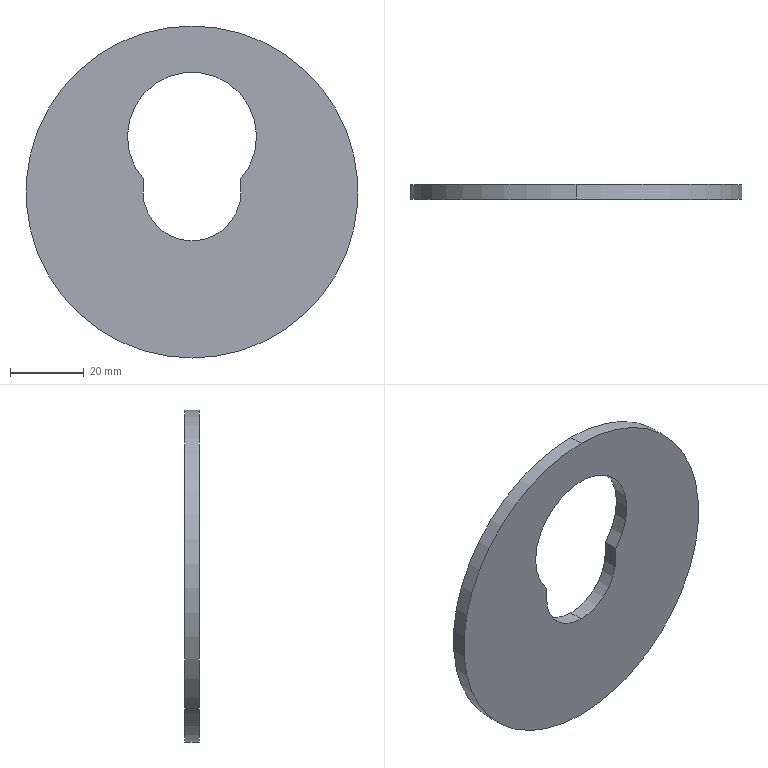Part | SolidWorks | features Extrusion 1, ICE 1 | 1 solid | 9 faces | box 90 x 4 x 90 mm | volume 20564 mm3 | cylinder 5 | plane 4 | commonest cylinder face diameters 26.5 x2 90 x2 35 x1
STEP:
#1=CARTESIAN_POINT('',(13.238,2.,0.5547));
#2=VERTEX_POINT('',#1);
#3=CARTESIAN_POINT('',(0.,2.,-13.25));
#4=VERTEX_POINT('',#3);
#5=CARTESIAN_POINT('',(0.,2.,0.));
#6=DIRECTION('',(0.,1.,0.));
#7=DIRECTION('',(0.,0.,1.));
#8=AXIS2_PLACEMENT_3D('',#5,#6,#7);
#9=CIRCLE('',#8,13.25);
#10=EDGE_CURVE('',#2,#4,#9,.T.);
#11=ORIENTED_EDGE('',*,*,#10,.T.);
#12=CARTESIAN_POINT('',(0.,-2.,-13.25));
#13=VERTEX_POINT('',#12);
#14=CARTESIAN_POINT('',(0.,2.,-13.25));
#15=DIRECTION('',(0.,-1.,0.));
#16=VECTOR('',#15,1000.);
#17=LINE('',#14,#16);
#18=EDGE_CURVE('',#4,#13,#17,.T.);
#19=ORIENTED_EDGE('',*,*,#18,.T.);
#20=CARTESIAN_POINT('',(13.238,-2.,0.5547));
#21=VERTEX_POINT('',#20);
#22=CARTESIAN_POINT('',(0.,-2.,0.));
#23=DIRECTION('',(0.,1.,0.));
#24=DIRECTION('',(0.,0.,1.));
#25=AXIS2_PLACEMENT_3D('',#22,#23,#24);
#26=CIRCLE('',#25,13.25);
#27=EDGE_CURVE('',#21,#13,#26,.T.);
#28=ORIENTED_EDGE('',*,*,#27,.F.);
#29=CARTESIAN_POINT('',(13.238,2.,0.5547));
#30=DIRECTION('',(0.,1.,0.));
#31=VECTOR('',#30,1000.);
#32=LINE('',#29,#31);
#33=EDGE_CURVE('',#21,#2,#32,.T.);
#34=ORIENTED_EDGE('',*,*,#33,.T.);
#35=EDGE_LOOP('',(#11,#19,#28,#34));
#36=FACE_OUTER_BOUND('',#35,.T.);
#37=CARTESIAN_POINT('',(0.,2.,0.));
#38=DIRECTION('',(0.,-1.,0.));
#39=DIRECTION('',(0.,0.,-1.));
#40=AXIS2_PLACEMENT_3D('',#37,#38,#39);
#41=CYLINDRICAL_SURFACE('',#40,13.25);
#42=ADVANCED_FACE('',(#36),#41,.F.);
#43=CARTESIAN_POINT('',(0.,2.,45.));
#44=VERTEX_POINT('',#43);
#45=CARTESIAN_POINT('',(0.,2.,-45.));
#46=VERTEX_POINT('',#45);
#47=CARTESIAN_POINT('',(0.,2.,0.));
#48=DIRECTION('',(0.,1.,0.));
#49=DIRECTION('',(0.,0.,1.));
#50=AXIS2_PLACEMENT_3D('',#47,#48,#49);
#51=CIRCLE('',#50,45.);
#52=EDGE_CURVE('',#44,#46,#51,.T.);
#53=ORIENTED_EDGE('',*,*,#52,.F.);
#54=CARTESIAN_POINT('',(0.,-2.,45.));
#55=VERTEX_POINT('',#54);
#56=CARTESIAN_POINT('',(0.,2.,45.));
#57=DIRECTION('',(0.,-1.,0.));
#58=VECTOR('',#57,1000.);
#59=LINE('',#56,#58);
#60=EDGE_CURVE('',#44,#55,#59,.T.);
#61=ORIENTED_EDGE('',*,*,#60,.T.);
#62=CARTESIAN_POINT('',(0.,-2.,-45.));
#63=VERTEX_POINT('',#62);
#64=CARTESIAN_POINT('',(0.,-2.,0.));
#65=DIRECTION('',(0.,1.,0.));
#66=DIRECTION('',(0.,0.,1.));
#67=AXIS2_PLACEMENT_3D('',#64,#65,#66);
#68=CIRCLE('',#67,45.);
#69=EDGE_CURVE('',#55,#63,#68,.T.);
#70=ORIENTED_EDGE('',*,*,#69,.T.);
#71=CARTESIAN_POINT('',(0.,2.,-45.));
#72=DIRECTION('',(0.,-1.,0.));
#73=VECTOR('',#72,1000.);
#74=LINE('',#71,#73);
#75=EDGE_CURVE('',#46,#63,#74,.T.);
#76=ORIENTED_EDGE('',*,*,#75,.F.);
#77=EDGE_LOOP('',(#53,#61,#70,#76));
#78=FACE_OUTER_BOUND('',#77,.T.);
#79=CARTESIAN_POINT('',(0.,2.,0.));
#80=DIRECTION('',(0.,-1.,0.));
#81=DIRECTION('',(0.,0.,-1.));
#82=AXIS2_PLACEMENT_3D('',#79,#80,#81);
#83=CYLINDRICAL_SURFACE('',#82,45.);
#84=ADVANCED_FACE('',(#78),#83,.T.);
#85=CARTESIAN_POINT('',(13.238,2.,3.555));
#86=VERTEX_POINT('',#85);
#87=CARTESIAN_POINT('',(13.238,2.,0.5547));
#88=DIRECTION('',(0.,0.,1.));
#89=VECTOR('',#88,1000.);
#90=LINE('',#87,#89);
#91=EDGE_CURVE('',#2,#86,#90,.T.);
#92=ORIENTED_EDGE('',*,*,#91,.T.);
#93=CARTESIAN_POINT('',(-13.238,2.,3.555));
#94=VERTEX_POINT('',#93);
#95=CARTESIAN_POINT('',(0.,2.,15.));
#96=DIRECTION('',(0.,-1.,0.));
#97=DIRECTION('',(0.,0.,1.));
#98=AXIS2_PLACEMENT_3D('',#95,#96,#97);
#99=CIRCLE('',#98,17.5);
#100=EDGE_CURVE('',#86,#94,#99,.T.);
#101=ORIENTED_EDGE('',*,*,#100,.T.);
#102=CARTESIAN_POINT('',(-13.238,2.,0.5547));
#103=VERTEX_POINT('',#102);
#104=CARTESIAN_POINT('',(-13.238,2.,0.5547));
#105=DIRECTION('',(0.,0.,-1.));
#106=VECTOR('',#105,1000.);
#107=LINE('',#104,#106);
#108=EDGE_CURVE('',#94,#103,#107,.T.);
#109=ORIENTED_EDGE('',*,*,#108,.T.);
#110=CARTESIAN_POINT('',(0.,2.,0.));
#111=DIRECTION('',(0.,1.,0.));
#112=DIRECTION('',(0.,0.,1.));
#113=AXIS2_PLACEMENT_3D('',#110,#111,#112);
#114=CIRCLE('',#113,13.25);
#115=EDGE_CURVE('',#4,#103,#114,.T.);
#116=ORIENTED_EDGE('',*,*,#115,.F.);
#117=ORIENTED_EDGE('',*,*,#10,.F.);
#118=EDGE_LOOP('',(#92,#101,#109,#116,#117));
#119=FACE_BOUND('',#118,.T.);
#120=CARTESIAN_POINT('',(0.,2.,0.));
#121=DIRECTION('',(0.,1.,0.));
#122=DIRECTION('',(0.,0.,1.));
#123=AXIS2_PLACEMENT_3D('',#120,#121,#122);
#124=CIRCLE('',#123,45.);
#125=EDGE_CURVE('',#46,#44,#124,.T.);
#126=ORIENTED_EDGE('',*,*,#125,.T.);
#127=ORIENTED_EDGE('',*,*,#52,.T.);
#128=EDGE_LOOP('',(#126,#127));
#129=FACE_OUTER_BOUND('',#128,.T.);
#130=CARTESIAN_POINT('',(0.,2.,0.));
#131=DIRECTION('',(0.,1.,0.));
#132=DIRECTION('',(0.,0.,1.));
#133=AXIS2_PLACEMENT_3D('',#130,#131,#132);
#134=PLANE('',#133);
#135=ADVANCED_FACE('',(#119,#129),#134,.T.);
#136=CARTESIAN_POINT('',(0.,-2.,0.));
#137=DIRECTION('',(0.,1.,0.));
#138=DIRECTION('',(0.,0.,1.));
#139=AXIS2_PLACEMENT_3D('',#136,#137,#138);
#140=CIRCLE('',#139,45.);
#141=EDGE_CURVE('',#63,#55,#140,.T.);
#142=ORIENTED_EDGE('',*,*,#141,.F.);
#143=ORIENTED_EDGE('',*,*,#69,.F.);
#144=EDGE_LOOP('',(#142,#143));
#145=FACE_OUTER_BOUND('',#144,.T.);
#146=CARTESIAN_POINT('',(13.238,-2.,3.555));
#147=VERTEX_POINT('',#146);
#148=CARTESIAN_POINT('',(-13.238,-2.,3.555));
#149=VERTEX_POINT('',#148);
#150=CARTESIAN_POINT('',(0.,-2.,15.));
#151=DIRECTION('',(0.,-1.,0.));
#152=DIRECTION('',(0.,0.,-1.));
#153=AXIS2_PLACEMENT_3D('',#150,#151,#152);
#154=CIRCLE('',#153,17.5);
#155=EDGE_CURVE('',#147,#149,#154,.T.);
#156=ORIENTED_EDGE('',*,*,#155,.F.);
#157=CARTESIAN_POINT('',(13.238,-2.,0.5547));
#158=DIRECTION('',(0.,0.,1.));
#159=VECTOR('',#158,1000.);
#160=LINE('',#157,#159);
#161=EDGE_CURVE('',#21,#147,#160,.T.);
#162=ORIENTED_EDGE('',*,*,#161,.F.);
#163=ORIENTED_EDGE('',*,*,#27,.T.);
#164=CARTESIAN_POINT('',(-13.238,-2.,0.5547));
#165=VERTEX_POINT('',#164);
#166=CARTESIAN_POINT('',(0.,-2.,0.));
#167=DIRECTION('',(0.,1.,0.));
#168=DIRECTION('',(0.,0.,1.));
#169=AXIS2_PLACEMENT_3D('',#166,#167,#168);
#170=CIRCLE('',#169,13.25);
#171=EDGE_CURVE('',#13,#165,#170,.T.);
#172=ORIENTED_EDGE('',*,*,#171,.T.);
#173=CARTESIAN_POINT('',(-13.238,-2.,0.5547));
#174=DIRECTION('',(0.,0.,-1.));
#175=VECTOR('',#174,1000.);
#176=LINE('',#173,#175);
#177=EDGE_CURVE('',#149,#165,#176,.T.);
#178=ORIENTED_EDGE('',*,*,#177,.F.);
#179=EDGE_LOOP('',(#156,#162,#163,#172,#178));
#180=FACE_BOUND('',#179,.T.);
#181=CARTESIAN_POINT('',(0.,-2.,0.));
#182=DIRECTION('',(0.,1.,0.));
#183=DIRECTION('',(0.,0.,1.));
#184=AXIS2_PLACEMENT_3D('',#181,#182,#183);
#185=PLANE('',#184);
#186=ADVANCED_FACE('',(#145,#180),#185,.F.);
#187=ORIENTED_EDGE('',*,*,#60,.F.);
#188=ORIENTED_EDGE('',*,*,#125,.F.);
#189=ORIENTED_EDGE('',*,*,#75,.T.);
#190=ORIENTED_EDGE('',*,*,#141,.T.);
#191=EDGE_LOOP('',(#187,#188,#189,#190));
#192=FACE_OUTER_BOUND('',#191,.T.);
#193=CARTESIAN_POINT('',(0.,2.,0.));
#194=DIRECTION('',(0.,-1.,0.));
#195=DIRECTION('',(0.,0.,-1.));
#196=AXIS2_PLACEMENT_3D('',#193,#194,#195);
#197=CYLINDRICAL_SURFACE('',#196,45.);
#198=ADVANCED_FACE('',(#192),#197,.T.);
#199=ORIENTED_EDGE('',*,*,#18,.F.);
#200=ORIENTED_EDGE('',*,*,#115,.T.);
#201=CARTESIAN_POINT('',(-13.238,2.,0.5547));
#202=DIRECTION('',(0.,-1.,0.));
#203=VECTOR('',#202,1000.);
#204=LINE('',#201,#203);
#205=EDGE_CURVE('',#103,#165,#204,.T.);
#206=ORIENTED_EDGE('',*,*,#205,.T.);
#207=ORIENTED_EDGE('',*,*,#171,.F.);
#208=EDGE_LOOP('',(#199,#200,#206,#207));
#209=FACE_OUTER_BOUND('',#208,.T.);
#210=CARTESIAN_POINT('',(0.,2.,0.));
#211=DIRECTION('',(0.,-1.,0.));
#212=DIRECTION('',(0.,0.,-1.));
#213=AXIS2_PLACEMENT_3D('',#210,#211,#212);
#214=CYLINDRICAL_SURFACE('',#213,13.25);
#215=ADVANCED_FACE('',(#209),#214,.F.);
#216=CARTESIAN_POINT('',(13.238,2.001,3.555));
#217=DIRECTION('',(0.,-1.,0.));
#218=VECTOR('',#217,1000.);
#219=LINE('',#216,#218);
#220=EDGE_CURVE('',#86,#147,#219,.T.);
#221=ORIENTED_EDGE('',*,*,#220,.T.);
#222=ORIENTED_EDGE('',*,*,#155,.T.);
#223=CARTESIAN_POINT('',(-13.238,2.001,3.555));
#224=DIRECTION('',(0.,-1.,0.));
#225=VECTOR('',#224,1000.);
#226=LINE('',#223,#225);
#227=EDGE_CURVE('',#94,#149,#226,.T.);
#228=ORIENTED_EDGE('',*,*,#227,.F.);
#229=ORIENTED_EDGE('',*,*,#100,.F.);
#230=EDGE_LOOP('',(#221,#222,#228,#229));
#231=FACE_OUTER_BOUND('',#230,.T.);
#232=CARTESIAN_POINT('',(0.,2.001,15.));
#233=DIRECTION('',(0.,-1.,0.));
#234=DIRECTION('',(0.,0.,-1.));
#235=AXIS2_PLACEMENT_3D('',#232,#233,#234);
#236=CYLINDRICAL_SURFACE('',#235,17.5);
#237=ADVANCED_FACE('',(#231),#236,.F.);
#238=ORIENTED_EDGE('',*,*,#33,.F.);
#239=ORIENTED_EDGE('',*,*,#161,.T.);
#240=ORIENTED_EDGE('',*,*,#220,.F.);
#241=ORIENTED_EDGE('',*,*,#91,.F.);
#242=EDGE_LOOP('',(#238,#239,#240,#241));
#243=FACE_OUTER_BOUND('',#242,.T.);
#244=CARTESIAN_POINT('',(13.238,2.001,0.5547));
#245=DIRECTION('',(1.,0.,0.));
#246=DIRECTION('',(0.,0.,-1.));
#247=AXIS2_PLACEMENT_3D('',#244,#245,#246);
#248=PLANE('',#247);
#249=ADVANCED_FACE('',(#243),#248,.F.);
#250=ORIENTED_EDGE('',*,*,#227,.T.);
#251=ORIENTED_EDGE('',*,*,#177,.T.);
#252=ORIENTED_EDGE('',*,*,#205,.F.);
#253=ORIENTED_EDGE('',*,*,#108,.F.);
#254=EDGE_LOOP('',(#250,#251,#252,#253));
#255=FACE_OUTER_BOUND('',#254,.T.);
#256=CARTESIAN_POINT('',(-13.238,2.001,0.5547));
#257=DIRECTION('',(-1.,0.,0.));
#258=DIRECTION('',(0.,0.,1.));
#259=AXIS2_PLACEMENT_3D('',#256,#257,#258);
#260=PLANE('',#259);
#261=ADVANCED_FACE('',(#255),#260,.F.);
#262=CLOSED_SHELL('',(#42,#84,#135,#186,#198,#215,#237,#249,#261));
#263=MANIFOLD_SOLID_BREP('',#262);
#264=CARTESIAN_POINT('',(0.,0.,0.));
#265=DIRECTION('',(0.,0.,1.));
#266=DIRECTION('',(1.,0.,0.));
#267=AXIS2_PLACEMENT_3D('',#264,#265,#266);
#268=(LENGTH_UNIT()NAMED_UNIT(*)SI_UNIT(.MILLI.,.METRE.));
#269=UNCERTAINTY_MEASURE_WITH_UNIT(LENGTH_MEASURE(0.00001),#268,'','');
#270=(NAMED_UNIT(*)PLANE_ANGLE_UNIT()SI_UNIT($,.RADIAN.));
#271=(NAMED_UNIT(*)SI_UNIT($,.STERADIAN.)SOLID_ANGLE_UNIT());
#272=(GEOMETRIC_REPRESENTATION_CONTEXT(3)GLOBAL_UNCERTAINTY_ASSIGNED_CONTEXT((#269))GLOBAL_UNIT_ASSIGNED_CONTEXT((#268,#270,#271))REPRESENTATION_CONTEXT('',''));
#273=ADVANCED_BREP_SHAPE_REPRESENTATION('',(#263,#267),#272);